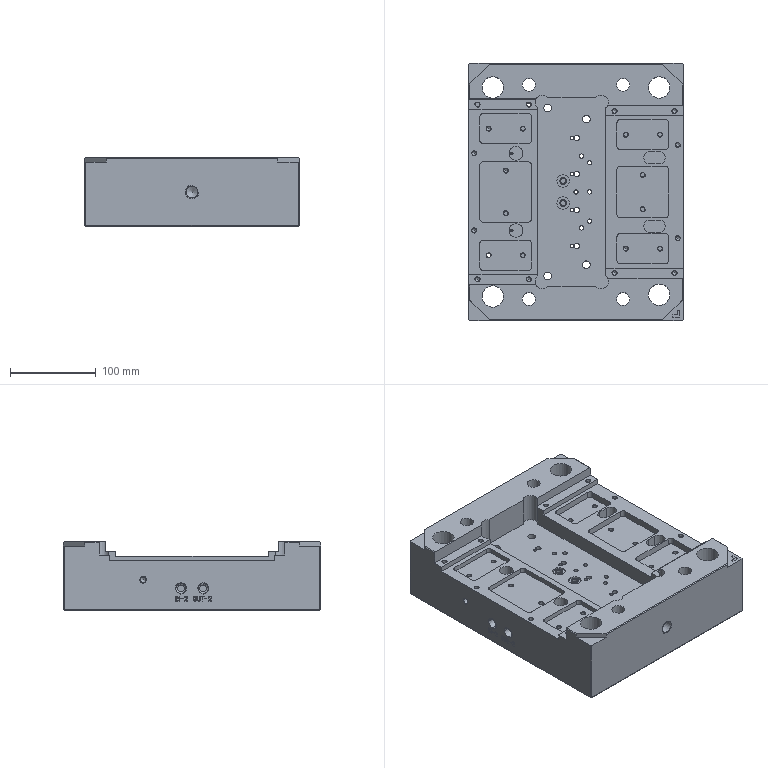NC program | PowerMill | posted with a generic post | part box 250 x 300 x 80 mm
Lines 1 to 740 of 72583:
%
O0001
N104 ( POWERMILL CB  : 2026004.0)
N105 ( POST VER      : 2026.0.0.5161)
N106 ( OPTION FILE   : FANUC)
N107 ( OUTPUT WORKPLANE : 1)
N108 (  )
N109 ( TOOL LIST )
N110 (---------------------------------------)
N111 ( NO. | ID        | DIA.| TIP RAD|LENGTH)
N112 (---------------------------------------)
N113 (    1|B17R0.8_1_1|17.0 |  0.8   |108.16)
N114 (---------------------------------------)
N115 (  )
N116 ( NUMBER OF TOOLPATHS: 1.0 )
N117 ( ESTIMATED PROGRAM DURATION: 0 HOURS 10 MIN 3 SEC)
N118 (  )
N119 G00 G21 G80 G40 G17
N120 G90
N121 G54
N122 G53 Z0.0
N123 (---------------)
N124 ( START TOOLPATH : 06中光-B17R0.8-等高 )
N125 (---------------)
N126 ( TOOL NO.    :1 )
N127 ( TOOL TYPE   : TIPRADIUSED)
N128 ( TOOL ID     : B17R0.8_1_1)
N129 ( TOOL DIA    : 17.0 LENGTH 108.16)
N130 T1
N131 M6
N132 S2200 M03
N133 G00 G90 X121.7482 Y-62.719
N134 G43 Z22.0 H1
N135
N136 G05 P10000 R8
N137 Z0.3
N138 G01 X122.383 Y-62.9767 Z0.2641 F2400.0
N139 X123.2071 Y-63.1887 Z0.2195
N140 X124.0313 Y-63.3421 Z0.1756
N141 X124.8554 Y-63.3928 Z0.1323
N142 X125.6795 Y-63.368 Z0.0891
N143 X126.5036 Y-63.2602 Z0.0455
N144 X127.3451 Y-63.0445 Z0.0
N145 X128.1519 Y-62.7736 F4000.0
N146 X128.976 Y-62.3811
N147 X129.2551 Y-62.2204
N148 X129.8002 Y-61.8704
N149 X130.6243 Y-61.2241
N150 X131.2598 Y-60.5722
N151 X131.4484 Y-60.353
N152 X131.9074 Y-59.748
N153 X132.4084 Y-58.9239
N154 X132.7883 Y-58.0998
N155 X133.0696 Y-57.2757
N156 X133.2614 Y-56.4515
N157 X133.3695 Y-55.6274
N158 X133.3847 Y-54.8033
N159 X133.3337 Y-53.9791
N160 X133.1774 Y-53.155
N161 X132.9587 Y-52.3309
N162 X132.6173 Y-51.5068
N163 X132.1945 Y-50.6826
N164 X131.9159 Y-50.2645
N165 X131.4484 Y-49.6453
N166 X130.8939 Y-49.0344
N167 X130.2776 Y-48.49
N168 X129.8002 Y-48.1228
N169 X128.976 Y-47.6163
N170 X128.1519 Y-47.2284
N171 X127.3278 Y-46.948
N172 X126.5036 Y-46.7488
N173 X125.6795 Y-46.634
N174 X124.8554 Y-46.6141
N175 X124.0313 Y-46.6641
N176 X123.2157 Y-46.8112
N177 X123.2071 Y-46.8037
N178 X122.383 Y-47.0287
N179 X121.494 Y-47.3861
N180 X120.7348 Y-47.7865
N181 X120.0773 Y-48.2102
N182 X119.5027 Y-48.6775
N183 X119.1134 Y-49.0344
N184 X118.7219 Y-49.451
N185 X118.2624 Y-50.0189
N186 X117.8118 Y-50.6826
N187 X117.3779 Y-51.5068
N188 X117.0486 Y-52.3309
N189 X116.827 Y-53.155
N190 X116.6778 Y-53.9791
N191 X116.609 Y-54.8033
N192 X116.6267 Y-55.6274
N193 X116.7316 Y-56.4515
N194 X116.9213 Y-57.2757
N195 X117.1994 Y-58.0998
N196 X117.5876 Y-58.9239
N197 X118.0951 Y-59.748
N198 X118.2624 Y-59.9881
N199 X118.738 Y-60.5722
N200 X119.0865 Y-60.9389
N201 X119.581 Y-61.3963
N202 X119.9106 Y-61.6704
N203 X120.7348 Y-62.2176
N204 X121.5589 Y-62.6422
N205 X122.383 Y-62.9767
N206 X123.2071 Y-63.1887
N207 X124.0313 Y-63.3421
N208 X124.8554 Y-63.3928
N209 X125.6795 Y-63.368
N210 X126.5036 Y-63.2602
N211 X127.3451 Y-63.0445
N212 X128.1467 Y-62.7615 Z-0.0033
N213 X128.5628 Y-62.5749 Z-0.005
N214 X129.2462 Y-62.2063 Z-0.008
N215 X129.7875 Y-61.8517 Z-0.0105
N216 X130.0999 Y-61.6235 Z-0.012
N217 X130.6 Y-61.1983 Z-0.0146
N218 X130.9292 Y-60.8805 Z-0.0163
N219 X131.4205 Y-60.3294 Z-0.0192
N220 X131.6541 Y-60.0325 Z-0.0206
N221 X132.06 Y-59.4361 Z-0.0234
N222 X132.3638 Y-58.9006 Z-0.0258
N223 X132.5655 Y-58.492 Z-0.0276
N224 X132.7401 Y-58.0706 Z-0.0293
N225 X133.008 Y-57.2608 Z-0.0326
N226 X133.1127 Y-56.852 Z-0.0343
N227 X133.2422 Y-56.0807 Z-0.0373
N228 X133.2835 Y-55.7226 Z-0.0387
N229 X133.3075 Y-55.2057 Z-0.0407
N230 X133.2787 Y-54.3723 Z-0.0439
N231 X133.2355 Y-53.9456 Z-0.0456
N232 X133.1682 Y-53.5319 Z-0.0472
N233 X132.966 Y-52.696 Z-0.0505
N234 X132.8633 Y-52.3631 Z-0.0519
N235 X132.7073 Y-51.9518 Z-0.0536
N236 X132.4836 Y-51.4457 Z-0.0557
N237 X132.1014 Y-50.7363 Z-0.0588
N238 X131.8313 Y-50.3196 Z-0.0607
N239 X131.3679 Y-49.7177 Z-0.0637
N240 X131.0588 Y-49.3663 Z-0.0655
N241 X130.5464 Y-48.8701 Z-0.0682
N242 X130.2052 Y-48.5782 Z-0.07
N243 X129.8822 Y-48.3323 Z-0.0715
N244 X129.5266 Y-48.0913 Z-0.0732
N245 X129.0464 Y-47.803 Z-0.0754
N246 X128.6254 Y-47.5848 Z-0.0772
N247 X128.2065 Y-47.3953 Z-0.079
N248 X127.8723 Y-47.2639 Z-0.0804
N249 X127.3673 Y-47.0985 Z-0.0824
N250 X126.8838 Y-46.9732 Z-0.0844
N251 X126.0695 Y-46.8265 Z-0.0876
N252 X125.6637 Y-46.7864 Z-0.0891
N253 X124.8471 Y-46.7662 Z-0.0923
N254 X124.4345 Y-46.7826 Z-0.0939
N255 X123.5987 Y-46.8922 Z-0.0972
N256 X123.1784 Y-46.9769 Z-0.0988
N257 X122.7618 Y-47.0823 Z-0.1005
N258 X122.1283 Y-47.2949 Z-0.1031
N259 X121.5165 Y-47.5568 Z-0.1057
N260 X121.099 Y-47.7674 Z-0.1075
N261 X120.4943 Y-48.1342 Z-0.1102
N262 X120.1689 Y-48.3578 Z-0.1117
N263 X119.8572 Y-48.6 Z-0.1133
N264 X119.4267 Y-48.9746 Z-0.1155
N265 X119.0256 Y-49.3757 Z-0.1177
N266 X118.6497 Y-49.8077 Z-0.1199
N267 X118.2012 Y-50.4163 Z-0.1228
N268 X117.7829 Y-51.1199 Z-0.126
N269 X117.6051 Y-51.4733 Z-0.1275
N270 X117.3748 Y-52.0112 Z-0.1298
N271 X117.2334 Y-52.3963 Z-0.1313
N272 X117.0161 Y-53.2004 Z-0.1346
N273 X116.8766 Y-53.9969 Z-0.1377
N274 X116.8247 Y-54.8104 Z-0.1408
N275 Y-55.2193 Z-0.1424
N276 X116.8476 Y-55.6277 Z-0.144
N277 X116.9612 Y-56.4633 Z-0.1473
N278 X117.0482 Y-56.8826 Z-0.1489
N279 X117.1594 Y-57.296 Z-0.1506
N280 X117.2968 Y-57.7092 Z-0.1523
N281 X117.4541 Y-58.1154 Z-0.1539
N282 X117.6423 Y-58.5355 Z-0.1557
N283 X117.8539 Y-58.9463 Z-0.1575
N284 X118.2817 Y-59.6257 Z-0.1606
N285 X118.7075 Y-60.1875 Z-0.1633
N286 X119.0649 Y-60.5893 Z-0.1654
N287 X119.4671 Y-60.9848 Z-0.1676
N288 X119.9712 Y-61.4135 Z-0.1702
N289 X120.4493 Y-61.7593 Z-0.1724
N290 X120.9932 Y-62.0931 Z-0.1749
N291 X121.5551 Y-62.3778 Z-0.1773
N292 X121.9622 Y-62.5547 Z-0.179
N293 X122.3799 Y-62.705 Z-0.1808
N294 X122.7889 Y-62.8293 Z-0.1824
N295 X123.615 Y-63.0181 Z-0.1857
N296 X124.4454 Y-63.1105 Z-0.1889
N297 X125.2708 Y-63.1265 Z-0.1921
N298 X126.0928 Y-63.0498 Z-0.1953
N299 X126.5039 Y-62.9835 Z-0.1969
N300 X127.2886 Y-62.8004 Z-0.2
N301 X128.2006 Y-62.4585 Z-0.2039
N302 X128.5896 Y-62.2801 Z-0.2055
N303 X128.9677 Y-62.08 Z-0.2072
N304 X129.3858 Y-61.825 Z-0.2092
N305 X130.0004 Y-61.3868 Z-0.2122
N306 X130.312 Y-61.1276 Z-0.2138
N307 X130.897 Y-60.5606 Z-0.217
N308 X131.1736 Y-60.255 Z-0.2186
N309 X131.574 Y-59.7365 Z-0.2212
N310 X131.8491 Y-59.3293 Z-0.2231
N311 X132.0967 Y-58.907 Z-0.2251
N312 X132.3718 Y-58.3551 Z-0.2275
N313 X132.6369 Y-57.6808 Z-0.2304
N314 X132.7709 Y-57.2657 Z-0.2321
N315 X132.8778 Y-56.8569 Z-0.2338
N316 X133.0216 Y-56.0356 Z-0.2371
N317 X133.065 Y-55.6271 Z-0.2387
N318 X133.085 Y-55.2163 Z-0.2403
N319 X133.0603 Y-54.3919 Z-0.2436
N320 X133.0165 Y-53.9563 Z-0.2453
N321 X132.95 Y-53.5406 Z-0.247
N322 X132.8597 Y-53.1296 Z-0.2487
N323 X132.7476 Y-52.7144 Z-0.2504
N324 X132.6113 Y-52.2943 Z-0.2521
N325 X132.4631 Y-51.9073 Z-0.2538
N326 X132.2909 Y-51.5305 Z-0.2554
N327 X132.0359 Y-51.0425 Z-0.2576
N328 X131.6039 Y-50.3577 Z-0.2608
N329 X131.2489 Y-49.8937 Z-0.2631
N330 X130.9749 Y-49.5753 Z-0.2647
N331 X130.4752 Y-49.0764 Z-0.2675
N332 X130.069 Y-48.7267 Z-0.2697
N333 X129.5086 Y-48.3175 Z-0.2724
N334 X128.9459 Y-47.9728 Z-0.275
N335 X128.5367 Y-47.7597 Z-0.2768
N336 X128.1248 Y-47.5726 Z-0.2786
N337 X127.7806 Y-47.4364 Z-0.2801
N338 X127.303 Y-47.2804 Z-0.2821
N339 X126.4868 Y-47.086 Z-0.2854
N340 X126.0805 Y-47.0183 Z-0.287
N341 X125.6705 Y-46.9768 Z-0.2887
N342 X124.8505 Y-46.9531 Z-0.2919
N343 X124.4352 Y-46.9692 Z-0.2936
N344 X124.0216 Y-47.0133 Z-0.2952
N345 X123.6025 Y-47.0784 Z-0.2969
N346 X123.1859 Y-47.1636 Z-0.2986
N347 X122.7736 Y-47.2688 Z-0.3003
N348 X122.3688 Y-47.4 Z-0.3019
N349 X121.9473 Y-47.5624 Z-0.3037
N350 X121.5326 Y-47.7481 Z-0.3055
N351 X121.137 Y-47.951 Z-0.3073
N352 X120.7608 Y-48.1693 Z-0.309
N353 X120.284 Y-48.4911 Z-0.3113
N354 X119.8806 Y-48.8035 Z-0.3133
N355 X119.5446 Y-49.1025 Z-0.3151
N356 X119.0542 Y-49.5974 Z-0.3178
N357 X118.7843 Y-49.9143 Z-0.3195
N358 X118.539 Y-50.2347 Z-0.3211
N359 X118.2461 Y-50.6622 Z-0.3231
N360 X117.9645 Y-51.1385 Z-0.3253
N361 X117.7566 Y-51.5452 Z-0.3271
N362 X117.5759 Y-51.9496 Z-0.3289
N363 X117.42 Y-52.3639 Z-0.3306
N364 X117.1902 Y-53.1742 Z-0.334
N365 X117.105 Y-53.5825 Z-0.3356
N366 X117.0414 Y-53.9949 Z-0.3373
N367 X116.9859 Y-54.8045 Z-0.3405
N368 X116.9851 Y-55.2164 Z-0.3421
N369 X117.0074 Y-55.6277 Z-0.3437
N370 X117.1206 Y-56.4552 Z-0.347
N371 X117.2081 Y-56.8719 Z-0.3487
N372 X117.3181 Y-57.2834 Z-0.3504
N373 X117.6199 Y-58.1099 Z-0.3539
N374 X117.8127 Y-58.5309 Z-0.3557
N375 X118.0245 Y-58.934 Z-0.3575
N376 X118.2483 Y-59.3082 Z-0.3593
N377 X118.5575 Y-59.7569 Z-0.3614
N378 X119.0742 Y-60.3784 Z-0.3646
N379 X119.262 Y-60.5822 Z-0.3657
N380 X119.5779 Y-60.8847 Z-0.3674
N381 X120.2083 Y-61.4073 Z-0.3707
N382 X120.728 Y-61.7619 Z-0.3732
N383 X121.1348 Y-62.0027 Z-0.375
N384 X121.6167 Y-62.2468 Z-0.3772
N385 X121.9937 Y-62.4117 Z-0.3788
N386 X122.38 Y-62.553 Z-0.3804
N387 X122.8267 Y-62.6919 Z-0.3823
N388 X123.6347 Y-62.8782 Z-0.3855
N389 X124.4529 Y-62.9708 Z-0.3888
N390 X125.2681 Y-62.9879 Z-0.392
N391 X126.093 Y-62.9112 Z-0.3953
N392 X126.8816 Y-62.7637 Z-0.3985
N393 X127.2539 Y-62.6597 Z-0.4
N394 X127.7689 Y-62.4876 Z-0.4022
N395 X128.4137 Y-62.218 Z-0.405
N396 X128.9733 Y-61.9254 Z-0.4075
N397 X129.3842 Y-61.671 Z-0.4094
N398 X130.0247 Y-61.197 Z-0.4126
N399 X130.7193 Y-60.5644 Z-0.4164
N400 X131.0866 Y-60.1585 Z-0.4186
N401 X131.4171 Y-59.7404 Z-0.4207
N402 X131.6959 Y-59.3349 Z-0.4227
N403 X131.9465 Y-58.9156 Z-0.4246
N404 X132.2581 Y-58.3034 Z-0.4274
N405 X132.5063 Y-57.6807 Z-0.4301
N406 X132.6427 Y-57.269 Z-0.4318
N407 X132.7502 Y-56.8604 Z-0.4335
N408 X132.8992 Y-56.0378 Z-0.4369
N409 X132.9442 Y-55.6266 Z-0.4385
N410 X132.9648 Y-55.215 Z-0.4402
N411 X132.94 Y-54.3818 Z-0.4435
N412 X132.8976 Y-53.9621 Z-0.4452
N413 X132.832 Y-53.5479 Z-0.4469
N414 X132.7414 Y-53.1383 Z-0.4486
N415 X132.6296 Y-52.7271 Z-0.4503
N416 X132.3779 Y-52.0076 Z-0.4533
N417 X132.1423 Y-51.4829 Z-0.4556
N418 X131.9162 Y-51.0614 Z-0.4576
N419 X131.6667 Y-50.6555 Z-0.4595
N420 X131.2407 Y-50.0603 Z-0.4624
N421 X130.8285 Y-49.5818 Z-0.4649
N422 X130.2207 Y-48.9994 Z-0.4683
N423 X129.7771 Y-48.6413 Z-0.4706
N424 X129.1946 Y-48.241 Z-0.4734
N425 X128.5485 Y-47.8846 Z-0.4764
N426 X128.1366 Y-47.6924 Z-0.4782
N427 X127.7314 Y-47.5314 Z-0.4799
N428 X127.317 Y-47.3959 Z-0.4817
N429 X126.9078 Y-47.2847 Z-0.4834
N430 X126.086 Y-47.1236 Z-0.4867
N431 X125.2669 Y-47.0593 Z-0.49
N432 X124.4322 Y-47.0722 Z-0.4934
N433 X124.0225 Y-47.1154 Z-0.495
N434 X123.2026 Y-47.2631 Z-0.4984
N435 X122.8206 Y-47.3591 Z-0.5
N436 X122.3675 Y-47.505 Z-0.5019
N437 X121.9511 Y-47.6675 Z-0.5037
N438 X121.2277 Y-48.0119 Z-0.5069
N439 X120.7205 Y-48.3124 Z-0.5092
N440 X120.2937 Y-48.6057 Z-0.5113
N441 X119.8946 Y-48.9192 Z-0.5133
N442 X119.4119 Y-49.3638 Z-0.516
N443 X119.0732 Y-49.7207 Z-0.5179
N444 X118.8335 Y-50.0017 Z-0.5194
N445 X118.6102 Y-50.2959 Z-0.5209
N446 X118.3246 Y-50.7121 Z-0.5229
N447 X118.0828 Y-51.1146 Z-0.5248
N448 X117.8658 Y-51.5273 Z-0.5267
N449 X117.681 Y-51.9325 Z-0.5285
N450 X117.4224 Y-52.6579 Z-0.5315
N451 X117.2835 Y-53.1687 Z-0.5337
N452 X117.1965 Y-53.5755 Z-0.5353
N453 X117.1326 Y-53.9867 Z-0.537
N454 X117.0738 Y-54.8038 Z-0.5403
N455 X117.0727 Y-55.2185 Z-0.5419
N456 X117.0947 Y-55.6327 Z-0.5436
N457 X117.2098 Y-56.4638 Z-0.547
N458 X117.2969 Y-56.8732 Z-0.5486
N459 X117.4045 Y-57.2776 Z-0.5503
N460 X117.5456 Y-57.6945 Z-0.5521
N461 X117.7085 Y-58.1038 Z-0.5539
N462 X117.9017 Y-58.522 Z-0.5557
N463 X118.118 Y-58.9288 Z-0.5575
N464 X118.3182 Y-59.2645 Z-0.5591
N465 X118.6613 Y-59.7579 Z-0.5615
N466 X119.1349 Y-60.3248 Z-0.5645
N467 X119.3735 Y-60.5801 Z-0.5659
N468 X119.9518 Y-61.103 Z-0.569
N469 X120.3389 Y-61.4032 Z-0.571
N470 X120.771 Y-61.6961 Z-0.5731
N471 X121.1733 Y-61.9348 Z-0.5749
N472 X121.6117 Y-62.1601 Z-0.5769
N473 X121.9927 Y-62.3271 Z-0.5786
N474 X122.3824 Y-62.4725 Z-0.5802
N475 X122.8104 Y-62.6082 Z-0.582
N476 X123.223 Y-62.716 Z-0.5837
N477 X123.6286 Y-62.8008 Z-0.5854
N478 X124.4462 Y-62.8959 Z-0.5887
N479 X125.2699 Y-62.9145 Z-0.592
N480 X126.0927 Y-62.8379 Z-0.5953
N481 X126.8771 Y-62.6914 Z-0.5985
N482 X127.237 Y-62.5909 Z-0.6
N483 X127.767 Y-62.4132 Z-0.6023
N484 X128.2402 Y-62.218 Z-0.6043
N485 X128.6168 Y-62.0365 Z-0.606
N486 X128.9966 Y-61.8296 Z-0.6077
N487 X129.3354 Y-61.6204 Z-0.6093
N488 X129.813 Y-61.2825 Z-0.6117
N489 X130.226 Y-60.9417 Z-0.6139
N490 X130.6435 Y-60.5461 Z-0.6162
N491 X130.9977 Y-60.1612 Z-0.6183
N492 X131.4636 Y-59.557 Z-0.6214
N493 X131.676 Y-59.245 Z-0.6229
N494 X132.0782 Y-58.5245 Z-0.6262
N495 X132.2901 Y-58.0611 Z-0.6283
N496 X132.4428 Y-57.6708 Z-0.63
N497 X132.5764 Y-57.2737 Z-0.6316
N498 X132.685 Y-56.8627 Z-0.6334
N499 X132.7721 Y-56.4466 Z-0.6351
N500 X132.8829 Y-55.6271 Z-0.6384
N501 X132.904 Y-55.215 Z-0.6401
N502 X132.8806 Y-54.389 Z-0.6434
N503 X132.8377 Y-53.9643 Z-0.6451
N504 X132.773 Y-53.5527 Z-0.6468
N505 X132.683 Y-53.1458 Z-0.6485
N506 X132.5697 Y-52.7301 Z-0.6502
N507 X132.4355 Y-52.3208 Z-0.6519
N508 X132.2625 Y-51.8789 Z-0.6539
N509 X132.0854 Y-51.4951 Z-0.6556
N510 X131.86 Y-51.0761 Z-0.6575
N511 X131.4364 Y-50.4149 Z-0.6606
N512 X131.2201 Y-50.1239 Z-0.6621
N513 X130.9877 Y-49.8456 Z-0.6636
N514 X130.3957 Y-49.2258 Z-0.667
N515 X129.7914 Y-48.7193 Z-0.6702
N516 X129.4181 Y-48.4516 Z-0.6721
N517 X128.968 Y-48.1697 Z-0.6742
N518 X128.556 Y-47.9456 Z-0.6761
N519 X128.1343 Y-47.7466 Z-0.678
N520 X127.733 Y-47.5867 Z-0.6797
N521 X127.0807 Y-47.3786 Z-0.6825
N522 X126.4924 Y-47.2435 Z-0.6849
N523 X126.0847 Y-47.1729 Z-0.6866
N524 X125.2674 Y-47.1076 Z-0.6899
N525 X124.4387 Y-47.1193 Z-0.6932
N526 X124.0244 Y-47.1625 Z-0.6949
N527 X123.6103 Y-47.2271 Z-0.6966
N528 X122.8329 Y-47.4033 Z-0.6998
N529 X122.3749 Y-47.5503 Z-0.7017
N530 X121.9583 Y-47.713 Z-0.7035
N531 X121.2392 Y-48.0562 Z-0.7068
N532 X120.7321 Y-48.3571 Z-0.7091
N533 X120.3043 Y-48.652 Z-0.7112
N534 X119.9082 Y-48.9642 Z-0.7133
N535 X119.4455 Y-49.3897 Z-0.7158
N536 X118.8748 Y-50.0168 Z-0.7192
N537 X118.3844 Y-50.6937 Z-0.7226
N538 X118.0821 Y-51.199 Z-0.725
N539 X117.9108 Y-51.524 Z-0.7264
N540 X117.726 Y-51.9259 Z-0.7282
N541 X117.5678 Y-52.3388 Z-0.73
N542 X117.4358 Y-52.7464 Z-0.7317
N543 X117.3242 Y-53.1608 Z-0.7335
N544 X117.2352 Y-53.5702 Z-0.7351
N545 X117.1705 Y-53.9842 Z-0.7368
N546 X117.1101 Y-54.8035 Z-0.7401
N547 X117.1086 Y-55.216 Z-0.7418
N548 X117.13 Y-55.628 Z-0.7435
N549 X117.2429 Y-56.4521 Z-0.7468
N550 X117.3306 Y-56.8665 Z-0.7485
N551 X117.4392 Y-57.2757 Z-0.7502
N552 X117.5802 Y-57.6919 Z-0.752
N553 X117.7454 Y-58.1061 Z-0.7538
N554 X117.9393 Y-58.524 Z-0.7557
N555 X118.2806 Y-59.1398 Z-0.7585
N556 X118.6992 Y-59.7553 Z-0.7615
N557 X119.1042 Y-60.2459 Z-0.7641
N558 X119.4162 Y-60.5793 Z-0.7659
N559 X119.9251 Y-61.0426 Z-0.7687
N560 X120.3848 Y-61.4002 Z-0.771
N561 X120.7497 Y-61.6493 Z-0.7728
N562 X121.1528 Y-61.8921 Z-0.7747
N563 X121.5704 Y-62.1101 Z-0.7766
N564 X122.1018 Y-62.3429 Z-0.7789
N565 X122.8046 Y-62.5789 Z-0.7819
N566 X123.2112 Y-62.6867 Z-0.7836
N567 X123.6223 Y-62.7731 Z-0.7853
N568 X124.4439 Y-62.8706 Z-0.7886
N569 X125.2707 Y-62.8902 Z-0.792
N570 X126.0989 Y-62.8133 Z-0.7953
N571 X126.8756 Y-62.6684 Z-0.7985
N572 X127.2307 Y-62.5654 Z-0.8
N573 X127.7588 Y-62.3927 Z-0.8022
N574 X128.1813 Y-62.2204 Z-0.8041
N575 X128.5842 Y-62.0297 Z-0.8059
N576 X128.976 Y-61.8179 Z-0.8077
N577 X129.3038 Y-61.6158 Z-0.8092
N578 X129.8002 Y-61.2672 Z-0.8117
N579 X130.2064 Y-60.9331 Z-0.8138
N580 X130.6243 Y-60.5385 Z-0.8161
N581 X130.9781 Y-60.1551 Z-0.8182
N582 X131.4484 Y-59.5474 Z-0.8213
N583 X131.6571 Y-59.242 Z-0.8228
N584 X132.0627 Y-58.5177 Z-0.8262
N585 X132.2725 Y-58.0602 Z-0.8282
N586 X132.4255 Y-57.6713 Z-0.8299
N587 X132.5594 Y-57.2757 Z-0.8316
N588 X132.668 Y-56.8662 Z-0.8333
N589 X132.7556 Y-56.4515 Z-0.835
N590 X132.8682 Y-55.6274 Z-0.8383
N591 X132.8896 Y-55.2156 Z-0.84
N592 X132.8669 Y-54.3904 Z-0.8433
N593 X132.8265 Y-53.9791 Z-0.845
N594 X132.7616 Y-53.5648 Z-0.8467
N595 X132.672 Y-53.155 Z-0.8484
N596 X132.5596 Y-52.7398 Z-0.8501
N597 X132.4263 Y-52.3309 Z-0.8519
N598 X132.2725 Y-51.9297 Z-0.8536
N599 X132.0779 Y-51.5068 Z-0.8555
N600 X131.8536 Y-51.088 Z-0.8574
N601 X131.4484 Y-50.4493 Z-0.8604
N602 X130.985 Y-49.8585 Z-0.8635
N603 X130.4009 Y-49.2436 Z-0.8669
N604 X129.8002 Y-48.7379 Z-0.8701
N605 X129.4184 Y-48.4627 Z-0.872
N606 X129.0215 Y-48.2103 Z-0.8739
N607 X128.5697 Y-47.9616 Z-0.8759
N608 X128.1519 Y-47.7626 Z-0.8778
N609 X127.7441 Y-47.5998 Z-0.8796
N610 X127.079 Y-47.3861 Z-0.8824
N611 X126.5036 Y-47.253 Z-0.8848
N612 X126.0936 Y-47.1815 Z-0.8865
N613 X125.2678 Y-47.1144 Z-0.8898
N614 X124.4424 Y-47.1253 Z-0.8931
N615 X124.0313 Y-47.168 Z-0.8948
N616 X123.6175 Y-47.2318 Z-0.8965
N617 X122.921 Y-47.3861 Z-0.8994
N618 X122.383 Y-47.5534 Z-0.9016
N619 X121.9665 Y-47.7153 Z-0.9034
N620 X121.2647 Y-48.0473 Z-0.9066
N621 X120.7348 Y-48.3608 Z-0.9091
N622 X120.3126 Y-48.6511 Z-0.9111
N623 X119.9106 Y-48.9676 Z-0.9132
N624 X119.4484 Y-49.3924 Z-0.9157
N625 X118.8829 Y-50.0129 Z-0.9191
N626 X118.3954 Y-50.6826 Z-0.9224
N627 X118.0874 Y-51.1959 Z-0.9249
N628 X117.9221 Y-51.5068 Z-0.9263
N629 X117.7348 Y-51.9134 Z-0.9281
N630 X117.5737 Y-52.3309 Z-0.9299
N631 X117.4382 Y-52.7471 Z-0.9317
N632 X117.328 Y-53.155 Z-0.9334
N633 X117.2384 Y-53.5648 Z-0.9351
N634 X117.1735 Y-53.9792 Z-0.9367
N635 X117.1121 Y-54.8033 Z-0.9401
N636 X117.1104 Y-55.2156 Z-0.9417
N637 X117.1318 Y-55.6274 Z-0.9434
N638 X117.2444 Y-56.4515 Z-0.9468
N639 X117.332 Y-56.8662 Z-0.9485
N640 X117.4406 Y-57.2757 Z-0.9502
N641 X117.5814 Y-57.6916 Z-0.952
N642 X117.744 Y-58.0998 Z-0.9537
N643 X117.9373 Y-58.5177 Z-0.9556
N644 X118.2624 Y-59.1072 Z-0.9583
N645 X118.6945 Y-59.748 Z-0.9614
N646 X119.0865 Y-60.2256 Z-0.9639
N647 X119.4095 Y-60.5721 Z-0.9658
N648 X119.9106 Y-61.0299 Z-0.9686
N649 X120.3801 Y-61.3963 Z-0.971
N650 X120.7348 Y-61.6396 Z-0.9727
N651 X121.1398 Y-61.8849 Z-0.9746
N652 X121.5589 Y-62.1042 Z-0.9765
N653 X122.0973 Y-62.341 Z-0.9789
N654 X122.7921 Y-62.5752 Z-0.9818
N655 X123.2071 Y-62.6857 Z-0.9836
N656 X123.6169 Y-62.7719 Z-0.9853
N657 X124.4427 Y-62.8705 Z-0.9886
N658 X125.268 Y-62.8902 Z-0.992
N659 X126.0929 Y-62.8141 Z-0.9953
N660 X126.8704 Y-62.6694 Z-0.9985
N661 X127.2307 Y-62.5654 Z-1.0
N662 X127.7588 Y-62.3927 Z-1.0022
N663 X128.1813 Y-62.2204 Z-1.0041
N664 X128.5842 Y-62.0297 Z-1.0059
N665 X128.976 Y-61.8179 Z-1.0077
N666 X129.3038 Y-61.6158 Z-1.0092
N667 X129.8002 Y-61.2672 Z-1.0117
N668 X130.2064 Y-60.9331 Z-1.0138
N669 X130.6243 Y-60.5385 Z-1.0161
N670 X130.9781 Y-60.1551 Z-1.0182
N671 X131.4484 Y-59.5474 Z-1.0213
N672 X131.6571 Y-59.242 Z-1.0228
N673 X132.0627 Y-58.5177 Z-1.0262
N674 X132.2725 Y-58.0602 Z-1.0282
N675 X132.4255 Y-57.6713 Z-1.0299
N676 X132.5594 Y-57.2757 Z-1.0316
N677 X132.668 Y-56.8662 Z-1.0333
N678 X132.7556 Y-56.4515 Z-1.035
N679 X132.8682 Y-55.6274 Z-1.0383
N680 X132.8896 Y-55.2156 Z-1.04
N681 X132.8669 Y-54.3904 Z-1.0433
N682 X132.8265 Y-53.9791 Z-1.045
N683 X132.7616 Y-53.5648 Z-1.0467
N684 X132.672 Y-53.155 Z-1.0484
N685 X132.5596 Y-52.7398 Z-1.0501
N686 X132.4263 Y-52.3309 Z-1.0519
N687 X132.2725 Y-51.9297 Z-1.0536
N688 X132.0779 Y-51.5068 Z-1.0555
N689 X131.8536 Y-51.088 Z-1.0574
N690 X131.4484 Y-50.4493 Z-1.0604
N691 X130.985 Y-49.8585 Z-1.0635
N692 X130.4009 Y-49.2436 Z-1.0669
N693 X129.8002 Y-48.7379 Z-1.0701
N694 X129.4184 Y-48.4627 Z-1.072
N695 X129.0215 Y-48.2103 Z-1.0739
N696 X128.5697 Y-47.9616 Z-1.0759
N697 X128.1519 Y-47.7626 Z-1.0778
N698 X127.7441 Y-47.5998 Z-1.0796
N699 X127.079 Y-47.3861 Z-1.0824
N700 X126.5036 Y-47.253 Z-1.0848
N701 X126.0936 Y-47.1815 Z-1.0865
N702 X125.2678 Y-47.1144 Z-1.0898
N703 X124.4424 Y-47.1253 Z-1.0931
N704 X124.0313 Y-47.168 Z-1.0948
N705 X123.6175 Y-47.2318 Z-1.0965
N706 X122.921 Y-47.3861 Z-1.0994
N707 X122.383 Y-47.5534 Z-1.1016
N708 X121.9665 Y-47.7153 Z-1.1034
N709 X121.2647 Y-48.0473 Z-1.1066
N710 X120.7348 Y-48.3608 Z-1.1091
N711 X120.3126 Y-48.6511 Z-1.1111
N712 X119.9106 Y-48.9676 Z-1.1132
N713 X119.4484 Y-49.3924 Z-1.1157
N714 X118.8829 Y-50.0129 Z-1.1191
N715 X118.3954 Y-50.6826 Z-1.1224
N716 X118.0874 Y-51.1959 Z-1.1249
N717 X117.9221 Y-51.5068 Z-1.1263
N718 X117.7348 Y-51.9134 Z-1.1281
N719 X117.5737 Y-52.3309 Z-1.1299
N720 X117.4382 Y-52.7471 Z-1.1317
N721 X117.328 Y-53.155 Z-1.1334
N722 X117.2384 Y-53.5648 Z-1.1351
N723 X117.1735 Y-53.9792 Z-1.1367
N724 X117.1121 Y-54.8033 Z-1.1401
N725 X117.1104 Y-55.2156 Z-1.1417
N726 X117.1318 Y-55.6274 Z-1.1434
N727 X117.2444 Y-56.4515 Z-1.1468
N728 X117.332 Y-56.8662 Z-1.1485
N729 X117.4406 Y-57.2757 Z-1.1502
N730 X117.5814 Y-57.6916 Z-1.152
N731 X117.744 Y-58.0998 Z-1.1537
N732 X117.9373 Y-58.5177 Z-1.1556
N733 X118.2624 Y-59.1072 Z-1.1583
N734 X118.6945 Y-59.748 Z-1.1614
N735 X119.0865 Y-60.2256 Z-1.1639
N736 X119.4095 Y-60.5721 Z-1.1658
N737 X119.9106 Y-61.0299 Z-1.1686
N738 X120.3801 Y-61.3963 Z-1.171
N739 X120.7348 Y-61.6396 Z-1.1727
N740 X121.1398 Y-61.8849 Z-1.1746
N741 X121.5589 Y-62.1042 Z-1.1765
N742 X122.0973 Y-62.341 Z-1.1789
N743 X122.7921 Y-62.5752 Z-1.1818
N744 X123.2071 Y-62.6857 Z-1.1836
N745 X123.6169 Y-62.7719 Z-1.1853
N746 X124.4427 Y-62.8705 Z-1.1886
N747 X125.268 Y-62.8902 Z-1.192
N748 X126.0929 Y-62.8141 Z-1.1953
N749 X126.8704 Y-62.6694 Z-1.1985
N750 X127.2307 Y-62.5654 Z-1.2
N751 X127.7588 Y-62.3927 Z-1.2022
N752 X128.1813 Y-62.2204 Z-1.2041
N753 X128.5842 Y-62.0297 Z-1.2059
N754 X128.976 Y-61.8179 Z-1.2077
N755 X129.3038 Y-61.6158 Z-1.2092
N756 X129.8002 Y-61.2672 Z-1.2117
N757 X130.2064 Y-60.9331 Z-1.2138
N758 X130.6243 Y-60.5385 Z-1.2161
N759 X130.9781 Y-60.1551 Z-1.2182
N760 X131.4484 Y-59.5474 Z-1.2213
N761 X131.6571 Y-59.242 Z-1.2228
N762 X132.0627 Y-58.5177 Z-1.2262
N763 X132.2725 Y-58.0602 Z-1.2282
N764 X132.4255 Y-57.6713 Z-1.2299
N765 X132.5594 Y-57.2757 Z-1.2316
N766 X132.668 Y-56.8662 Z-1.2333
N767 X132.7556 Y-56.4515 Z-1.235
N768 X132.8682 Y-55.6274 Z-1.2383
N769 X132.8896 Y-55.2156 Z-1.24
N770 X132.8669 Y-54.3904 Z-1.2433
N771 X132.8265 Y-53.9791 Z-1.245
N772 X132.7616 Y-53.5648 Z-1.2467
N773 X132.672 Y-53.155 Z-1.2484
N774 X132.5596 Y-52.7398 Z-1.2501
N775 X132.4263 Y-52.3309 Z-1.2519
N776 X132.2725 Y-51.9297 Z-1.2536
N777 X132.0779 Y-51.5068 Z-1.2555
N778 X131.8536 Y-51.088 Z-1.2574
N779 X131.4484 Y-50.4493 Z-1.2604
N780 X130.985 Y-49.8585 Z-1.2635
N781 X130.4009 Y-49.2436 Z-1.2669
N782 X129.8002 Y-48.7379 Z-1.2701
N783 X129.4184 Y-48.4627 Z-1.272
N784 X129.0215 Y-48.2103 Z-1.2739
N785 X128.5697 Y-47.9616 Z-1.2759
N786 X128.1519 Y-47.7626 Z-1.2778
N787 X127.7441 Y-47.5998 Z-1.2796
N788 X127.079 Y-47.3861 Z-1.2824
N789 X126.5036 Y-47.253 Z-1.2848
N790 X126.0936 Y-47.1815 Z-1.2865
N791 X125.2678 Y-47.1144 Z-1.2898
N792 X124.4424 Y-47.1253 Z-1.2931
N793 X124.0313 Y-47.168 Z-1.2948
N794 X123.6175 Y-47.2318 Z-1.2965
N795 X122.921 Y-47.3861 Z-1.2994
N796 X122.383 Y-47.5534 Z-1.3016
N797 X121.9665 Y-47.7153 Z-1.3034
N798 X121.2647 Y-48.0473 Z-1.3066
N799 X120.7348 Y-48.3608 Z-1.3091
N800 X120.3126 Y-48.6511 Z-1.3111
N801 X119.9106 Y-48.9676 Z-1.3132
N802 X119.4484 Y-49.3924 Z-1.3157
N803 X118.8829 Y-50.0129 Z-1.3191
N804 X118.3954 Y-50.6826 Z-1.3224
N805 X118.0874 Y-51.1959 Z-1.3249
N806 X117.9221 Y-51.5068 Z-1.3263
N807 X117.7348 Y-51.9134 Z-1.3281
N808 X117.5737 Y-52.3309 Z-1.3299
N809 X117.4382 Y-52.7471 Z-1.3317
N810 X117.328 Y-53.155 Z-1.3334
N811 X117.2384 Y-53.5648 Z-1.3351
N812 X117.1735 Y-53.9792 Z-1.3367
N813 X117.1121 Y-54.8033 Z-1.3401
N814 X117.1104 Y-55.2156 Z-1.3417
N815 X117.1318 Y-55.6274 Z-1.3434
N816 X117.2444 Y-56.4515 Z-1.3468
N817 X117.332 Y-56.8662 Z-1.3485
N818 X117.4406 Y-57.2757 Z-1.3502
N819 X117.5814 Y-57.6916 Z-1.352
N820 X117.744 Y-58.0998 Z-1.3537
N821 X117.9373 Y-58.5177 Z-1.3556
N822 X118.2624 Y-59.1072 Z-1.3583
N823 X118.6945 Y-59.748 Z-1.3614
N824 X119.0865 Y-60.2256 Z-1.3639
N825 X119.4095 Y-60.5721 Z-1.3658
N826 X119.9106 Y-61.0299 Z-1.3686
N827 X120.3801 Y-61.3963 Z-1.371
N828 X120.7348 Y-61.6396 Z-1.3727
N829 X121.1398 Y-61.8849 Z-1.3746
N830 X121.5589 Y-62.1042 Z-1.3765
N831 X122.0973 Y-62.341 Z-1.3789
N832 X122.7921 Y-62.5752 Z-1.3818
N833 X123.2071 Y-62.6857 Z-1.3836
N834 X123.6169 Y-62.7719 Z-1.3853
N835 X124.4427 Y-62.8705 Z-1.3886
N836 X125.268 Y-62.8902 Z-1.392
N837 X126.0929 Y-62.8141 Z-1.3953